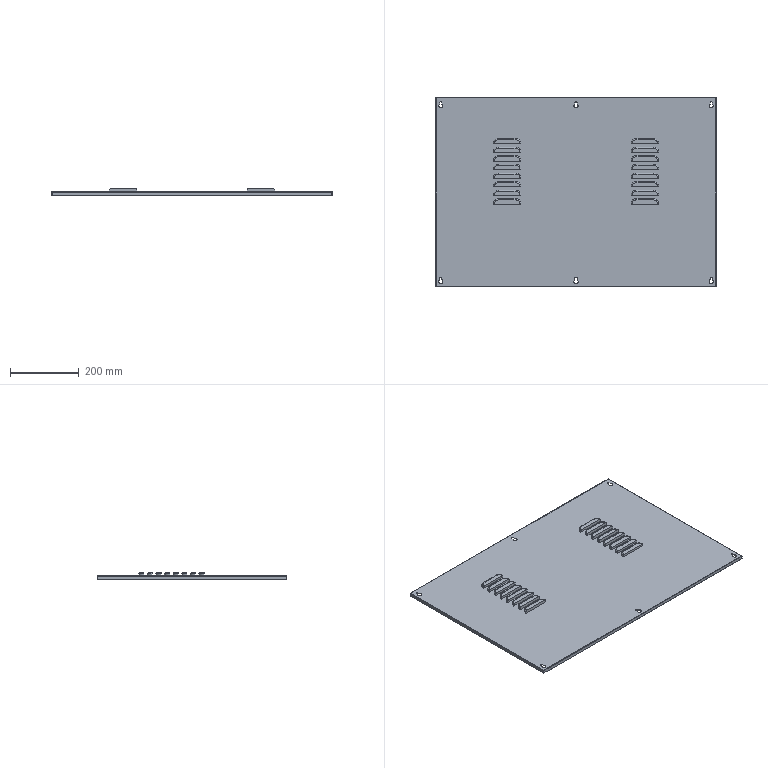Part | NX | features BREP 1 | 1 solid | 251 faces | box 815 x 550 x 18 mm | volume 845006 mm3 | cylinder 112 | plane 103 | torus 32 | sphere 4 | commonest cylinder face diameters 6 x54 28 x32 12 x18 2 x8